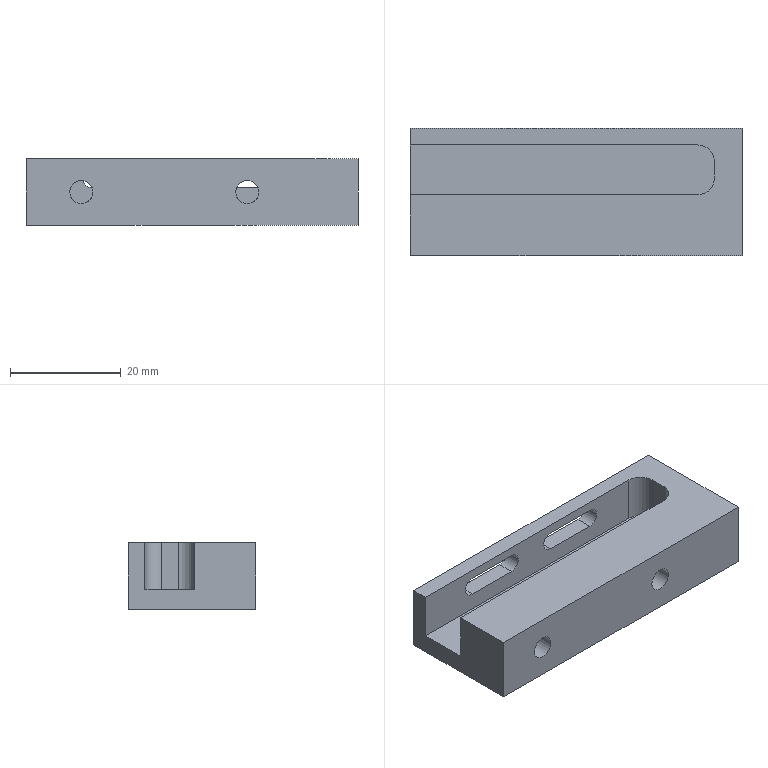Part | NX | features BREP 1 | 1 solid | 22 faces | box 60 x 23 x 12 mm | volume 11813 mm3 | plane 14 | cylinder 8 | commonest cylinder face diameters 3.5 x4 4.2 x2 6 x2
STEP:
#1=CARTESIAN_POINT('',(0.,-12.,6.));
#2=VERTEX_POINT('',#1);
#3=CARTESIAN_POINT('',(0.,-23.,6.));
#4=VERTEX_POINT('',#3);
#5=CARTESIAN_POINT('',(0.,0.,6.));
#6=DIRECTION('',(0.,-1.,0.));
#7=VECTOR('',#6,1000.);
#8=LINE('',#5,#7);
#9=EDGE_CURVE('',#2,#4,#8,.T.);
#10=ORIENTED_EDGE('',*,*,#9,.F.);
#11=CARTESIAN_POINT('',(0.,-12.,-2.5));
#12=VERTEX_POINT('',#11);
#13=CARTESIAN_POINT('',(0.,-12.,-2.5));
#14=DIRECTION('',(0.,0.,1.));
#15=VECTOR('',#14,1000.);
#16=LINE('',#13,#15);
#17=EDGE_CURVE('',#12,#2,#16,.T.);
#18=ORIENTED_EDGE('',*,*,#17,.F.);
#19=CARTESIAN_POINT('',(0.,-3.,-2.5));
#20=VERTEX_POINT('',#19);
#21=CARTESIAN_POINT('',(0.,0.,-2.5));
#22=DIRECTION('',(0.,-1.,0.));
#23=VECTOR('',#22,1000.);
#24=LINE('',#21,#23);
#25=EDGE_CURVE('',#20,#12,#24,.T.);
#26=ORIENTED_EDGE('',*,*,#25,.F.);
#27=CARTESIAN_POINT('',(0.,-3.,6.));
#28=VERTEX_POINT('',#27);
#29=CARTESIAN_POINT('',(0.,-3.,-2.5));
#30=DIRECTION('',(0.,0.,1.));
#31=VECTOR('',#30,1000.);
#32=LINE('',#29,#31);
#33=EDGE_CURVE('',#20,#28,#32,.T.);
#34=ORIENTED_EDGE('',*,*,#33,.T.);
#35=CARTESIAN_POINT('',(0.,0.,6.));
#36=VERTEX_POINT('',#35);
#37=CARTESIAN_POINT('',(0.,0.,6.));
#38=DIRECTION('',(0.,-1.,0.));
#39=VECTOR('',#38,1000.);
#40=LINE('',#37,#39);
#41=EDGE_CURVE('',#36,#28,#40,.T.);
#42=ORIENTED_EDGE('',*,*,#41,.F.);
#43=CARTESIAN_POINT('',(0.,0.,-6.));
#44=VERTEX_POINT('',#43);
#45=CARTESIAN_POINT('',(0.,0.,6.));
#46=DIRECTION('',(0.,0.,-1.));
#47=VECTOR('',#46,1000.);
#48=LINE('',#45,#47);
#49=EDGE_CURVE('',#36,#44,#48,.T.);
#50=ORIENTED_EDGE('',*,*,#49,.T.);
#51=CARTESIAN_POINT('',(0.,-23.,-6.));
#52=VERTEX_POINT('',#51);
#53=CARTESIAN_POINT('',(0.,0.,-6.));
#54=DIRECTION('',(0.,-1.,0.));
#55=VECTOR('',#54,1000.);
#56=LINE('',#53,#55);
#57=EDGE_CURVE('',#44,#52,#56,.T.);
#58=ORIENTED_EDGE('',*,*,#57,.T.);
#59=CARTESIAN_POINT('',(0.,-23.,6.));
#60=DIRECTION('',(0.,0.,-1.));
#61=VECTOR('',#60,1000.);
#62=LINE('',#59,#61);
#63=EDGE_CURVE('',#4,#52,#62,.T.);
#64=ORIENTED_EDGE('',*,*,#63,.F.);
#65=EDGE_LOOP('',(#10,#18,#26,#34,#42,#50,#58,#64));
#66=FACE_BOUND('',#65,.T.);
#67=CARTESIAN_POINT('',(0.,0.,6.));
#68=DIRECTION('',(1.,0.,0.));
#69=DIRECTION('',(0.,-1.,0.));
#70=AXIS2_PLACEMENT_3D('',#67,#68,#69);
#71=PLANE('',#70);
#72=ADVANCED_FACE('',(#66),#71,.F.);
#73=CARTESIAN_POINT('',(10.,-23.,-2.1));
#74=VERTEX_POINT('',#73);
#75=CARTESIAN_POINT('',(10.,-23.,0.));
#76=DIRECTION('',(0.,-1.,0.));
#77=DIRECTION('',(0.,0.,-1.));
#78=AXIS2_PLACEMENT_3D('',#75,#76,#77);
#79=CIRCLE('',#78,2.1);
#80=EDGE_CURVE('',#74,#74,#79,.T.);
#81=ORIENTED_EDGE('',*,*,#80,.F.);
#82=EDGE_LOOP('',(#81));
#83=FACE_BOUND('',#82,.T.);
#84=CARTESIAN_POINT('',(40.,-23.,-2.1));
#85=VERTEX_POINT('',#84);
#86=CARTESIAN_POINT('',(40.,-23.,0.));
#87=DIRECTION('',(0.,-1.,0.));
#88=DIRECTION('',(0.,0.,-1.));
#89=AXIS2_PLACEMENT_3D('',#86,#87,#88);
#90=CIRCLE('',#89,2.1);
#91=EDGE_CURVE('',#85,#85,#90,.T.);
#92=ORIENTED_EDGE('',*,*,#91,.F.);
#93=EDGE_LOOP('',(#92));
#94=FACE_BOUND('',#93,.T.);
#95=CARTESIAN_POINT('',(60.,-23.,-6.));
#96=VERTEX_POINT('',#95);
#97=CARTESIAN_POINT('',(0.,-23.,-6.));
#98=DIRECTION('',(1.,0.,0.));
#99=VECTOR('',#98,1000.);
#100=LINE('',#97,#99);
#101=EDGE_CURVE('',#52,#96,#100,.T.);
#102=ORIENTED_EDGE('',*,*,#101,.T.);
#103=CARTESIAN_POINT('',(60.,-23.,6.));
#104=VERTEX_POINT('',#103);
#105=CARTESIAN_POINT('',(60.,-23.,6.));
#106=DIRECTION('',(0.,0.,-1.));
#107=VECTOR('',#106,1000.);
#108=LINE('',#105,#107);
#109=EDGE_CURVE('',#104,#96,#108,.T.);
#110=ORIENTED_EDGE('',*,*,#109,.F.);
#111=CARTESIAN_POINT('',(0.,-23.,6.));
#112=DIRECTION('',(1.,0.,0.));
#113=VECTOR('',#112,1000.);
#114=LINE('',#111,#113);
#115=EDGE_CURVE('',#4,#104,#114,.T.);
#116=ORIENTED_EDGE('',*,*,#115,.F.);
#117=ORIENTED_EDGE('',*,*,#63,.T.);
#118=EDGE_LOOP('',(#102,#110,#116,#117));
#119=FACE_BOUND('',#118,.T.);
#120=CARTESIAN_POINT('',(0.,-23.,6.));
#121=DIRECTION('',(0.,1.,0.));
#122=DIRECTION('',(0.,0.,-1.));
#123=AXIS2_PLACEMENT_3D('',#120,#121,#122);
#124=PLANE('',#123);
#125=ADVANCED_FACE('',(#83,#94,#119),#124,.F.);
#126=CARTESIAN_POINT('',(60.,0.,-6.));
#127=VERTEX_POINT('',#126);
#128=CARTESIAN_POINT('',(60.,0.,-6.));
#129=DIRECTION('',(0.,1.,0.));
#130=VECTOR('',#129,1000.);
#131=LINE('',#128,#130);
#132=EDGE_CURVE('',#96,#127,#131,.T.);
#133=ORIENTED_EDGE('',*,*,#132,.T.);
#134=CARTESIAN_POINT('',(60.,0.,6.));
#135=VERTEX_POINT('',#134);
#136=CARTESIAN_POINT('',(60.,0.,6.));
#137=DIRECTION('',(0.,0.,-1.));
#138=VECTOR('',#137,1000.);
#139=LINE('',#136,#138);
#140=EDGE_CURVE('',#135,#127,#139,.T.);
#141=ORIENTED_EDGE('',*,*,#140,.F.);
#142=CARTESIAN_POINT('',(60.,0.,6.));
#143=DIRECTION('',(0.,1.,0.));
#144=VECTOR('',#143,1000.);
#145=LINE('',#142,#144);
#146=EDGE_CURVE('',#104,#135,#145,.T.);
#147=ORIENTED_EDGE('',*,*,#146,.F.);
#148=ORIENTED_EDGE('',*,*,#109,.T.);
#149=EDGE_LOOP('',(#133,#141,#147,#148));
#150=FACE_BOUND('',#149,.T.);
#151=CARTESIAN_POINT('',(60.,0.,6.));
#152=DIRECTION('',(-1.,0.,0.));
#153=DIRECTION('',(0.,0.,-1.));
#154=AXIS2_PLACEMENT_3D('',#151,#152,#153);
#155=PLANE('',#154);
#156=ADVANCED_FACE('',(#150),#155,.F.);
#157=CARTESIAN_POINT('',(32.,0.,0.75));
#158=VERTEX_POINT('',#157);
#159=CARTESIAN_POINT('',(32.,0.,4.25));
#160=VERTEX_POINT('',#159);
#161=CARTESIAN_POINT('',(32.,0.,2.5));
#162=DIRECTION('',(0.,1.,0.));
#163=DIRECTION('',(0.,0.,1.));
#164=AXIS2_PLACEMENT_3D('',#161,#162,#163);
#165=CIRCLE('',#164,1.75);
#166=EDGE_CURVE('',#158,#160,#165,.T.);
#167=ORIENTED_EDGE('',*,*,#166,.F.);
#168=CARTESIAN_POINT('',(42.,0.,0.75));
#169=VERTEX_POINT('',#168);
#170=CARTESIAN_POINT('',(42.,0.,0.75));
#171=DIRECTION('',(-1.,0.,0.));
#172=VECTOR('',#171,1000.);
#173=LINE('',#170,#172);
#174=EDGE_CURVE('',#169,#158,#173,.T.);
#175=ORIENTED_EDGE('',*,*,#174,.F.);
#176=CARTESIAN_POINT('',(42.,0.,4.25));
#177=VERTEX_POINT('',#176);
#178=CARTESIAN_POINT('',(42.,0.,2.5));
#179=DIRECTION('',(0.,1.,0.));
#180=DIRECTION('',(0.,0.,1.));
#181=AXIS2_PLACEMENT_3D('',#178,#179,#180);
#182=CIRCLE('',#181,1.75);
#183=EDGE_CURVE('',#177,#169,#182,.T.);
#184=ORIENTED_EDGE('',*,*,#183,.F.);
#185=CARTESIAN_POINT('',(42.,0.,4.25));
#186=DIRECTION('',(1.,0.,0.));
#187=VECTOR('',#186,1000.);
#188=LINE('',#185,#187);
#189=EDGE_CURVE('',#160,#177,#188,.T.);
#190=ORIENTED_EDGE('',*,*,#189,.F.);
#191=EDGE_LOOP('',(#167,#175,#184,#190));
#192=FACE_BOUND('',#191,.T.);
#193=CARTESIAN_POINT('',(12.,0.,0.75));
#194=VERTEX_POINT('',#193);
#195=CARTESIAN_POINT('',(12.,0.,4.25));
#196=VERTEX_POINT('',#195);
#197=CARTESIAN_POINT('',(12.,0.,2.5));
#198=DIRECTION('',(0.,1.,0.));
#199=DIRECTION('',(0.,0.,1.));
#200=AXIS2_PLACEMENT_3D('',#197,#198,#199);
#201=CIRCLE('',#200,1.75);
#202=EDGE_CURVE('',#194,#196,#201,.T.);
#203=ORIENTED_EDGE('',*,*,#202,.F.);
#204=CARTESIAN_POINT('',(22.,0.,0.75));
#205=VERTEX_POINT('',#204);
#206=CARTESIAN_POINT('',(22.,0.,0.75));
#207=DIRECTION('',(-1.,0.,0.));
#208=VECTOR('',#207,1000.);
#209=LINE('',#206,#208);
#210=EDGE_CURVE('',#205,#194,#209,.T.);
#211=ORIENTED_EDGE('',*,*,#210,.F.);
#212=CARTESIAN_POINT('',(22.,0.,4.25));
#213=VERTEX_POINT('',#212);
#214=CARTESIAN_POINT('',(22.,0.,2.5));
#215=DIRECTION('',(0.,1.,0.));
#216=DIRECTION('',(0.,0.,1.));
#217=AXIS2_PLACEMENT_3D('',#214,#215,#216);
#218=CIRCLE('',#217,1.75);
#219=EDGE_CURVE('',#213,#205,#218,.T.);
#220=ORIENTED_EDGE('',*,*,#219,.F.);
#221=CARTESIAN_POINT('',(22.,0.,4.25));
#222=DIRECTION('',(1.,0.,0.));
#223=VECTOR('',#222,1000.);
#224=LINE('',#221,#223);
#225=EDGE_CURVE('',#196,#213,#224,.T.);
#226=ORIENTED_EDGE('',*,*,#225,.F.);
#227=EDGE_LOOP('',(#203,#211,#220,#226));
#228=FACE_BOUND('',#227,.T.);
#229=CARTESIAN_POINT('',(0.,0.,-6.));
#230=DIRECTION('',(-1.,0.,0.));
#231=VECTOR('',#230,1000.);
#232=LINE('',#229,#231);
#233=EDGE_CURVE('',#127,#44,#232,.T.);
#234=ORIENTED_EDGE('',*,*,#233,.T.);
#235=ORIENTED_EDGE('',*,*,#49,.F.);
#236=CARTESIAN_POINT('',(0.,0.,6.));
#237=DIRECTION('',(-1.,0.,0.));
#238=VECTOR('',#237,1000.);
#239=LINE('',#236,#238);
#240=EDGE_CURVE('',#135,#36,#239,.T.);
#241=ORIENTED_EDGE('',*,*,#240,.F.);
#242=ORIENTED_EDGE('',*,*,#140,.T.);
#243=EDGE_LOOP('',(#234,#235,#241,#242));
#244=FACE_BOUND('',#243,.T.);
#245=CARTESIAN_POINT('',(0.,0.,6.));
#246=DIRECTION('',(0.,-1.,0.));
#247=DIRECTION('',(0.,0.,1.));
#248=AXIS2_PLACEMENT_3D('',#245,#246,#247);
#249=PLANE('',#248);
#250=ADVANCED_FACE('',(#192,#228,#244),#249,.F.);
#251=CARTESIAN_POINT('',(52.,-12.,6.));
#252=VERTEX_POINT('',#251);
#253=CARTESIAN_POINT('',(0.,-12.,6.));
#254=DIRECTION('',(1.,0.,0.));
#255=VECTOR('',#254,1000.);
#256=LINE('',#253,#255);
#257=EDGE_CURVE('',#2,#252,#256,.T.);
#258=ORIENTED_EDGE('',*,*,#257,.F.);
#259=ORIENTED_EDGE('',*,*,#9,.T.);
#260=ORIENTED_EDGE('',*,*,#115,.T.);
#261=ORIENTED_EDGE('',*,*,#146,.T.);
#262=ORIENTED_EDGE('',*,*,#240,.T.);
#263=ORIENTED_EDGE('',*,*,#41,.T.);
#264=CARTESIAN_POINT('',(52.,-3.,6.));
#265=VERTEX_POINT('',#264);
#266=CARTESIAN_POINT('',(0.,-3.,6.));
#267=DIRECTION('',(1.,0.,0.));
#268=VECTOR('',#267,1000.);
#269=LINE('',#266,#268);
#270=EDGE_CURVE('',#28,#265,#269,.T.);
#271=ORIENTED_EDGE('',*,*,#270,.T.);
#272=CARTESIAN_POINT('',(55.,-6.,6.));
#273=VERTEX_POINT('',#272);
#274=CARTESIAN_POINT('',(52.,-6.,6.));
#275=DIRECTION('',(0.,0.,-1.));
#276=DIRECTION('',(1.,0.,0.));
#277=AXIS2_PLACEMENT_3D('',#274,#275,#276);
#278=CIRCLE('',#277,3.);
#279=EDGE_CURVE('',#265,#273,#278,.T.);
#280=ORIENTED_EDGE('',*,*,#279,.T.);
#281=CARTESIAN_POINT('',(55.,-9.,6.));
#282=VERTEX_POINT('',#281);
#283=CARTESIAN_POINT('',(55.,0.,6.));
#284=DIRECTION('',(0.,-1.,0.));
#285=VECTOR('',#284,1000.);
#286=LINE('',#283,#285);
#287=EDGE_CURVE('',#273,#282,#286,.T.);
#288=ORIENTED_EDGE('',*,*,#287,.T.);
#289=CARTESIAN_POINT('',(52.,-9.,6.));
#290=DIRECTION('',(0.,0.,-1.));
#291=DIRECTION('',(1.,0.,0.));
#292=AXIS2_PLACEMENT_3D('',#289,#290,#291);
#293=CIRCLE('',#292,3.);
#294=EDGE_CURVE('',#282,#252,#293,.T.);
#295=ORIENTED_EDGE('',*,*,#294,.T.);
#296=EDGE_LOOP('',(#258,#259,#260,#261,#262,#263,#271,#280,#288,#295));
#297=FACE_BOUND('',#296,.T.);
#298=CARTESIAN_POINT('',(0.,0.,6.));
#299=DIRECTION('',(0.,0.,1.));
#300=DIRECTION('',(-1.,0.,0.));
#301=AXIS2_PLACEMENT_3D('',#298,#299,#300);
#302=PLANE('',#301);
#303=ADVANCED_FACE('',(#297),#302,.T.);
#304=ORIENTED_EDGE('',*,*,#57,.F.);
#305=ORIENTED_EDGE('',*,*,#233,.F.);
#306=ORIENTED_EDGE('',*,*,#132,.F.);
#307=ORIENTED_EDGE('',*,*,#101,.F.);
#308=EDGE_LOOP('',(#304,#305,#306,#307));
#309=FACE_BOUND('',#308,.T.);
#310=CARTESIAN_POINT('',(0.,0.,-6.));
#311=DIRECTION('',(0.,0.,1.));
#312=DIRECTION('',(-1.,0.,0.));
#313=AXIS2_PLACEMENT_3D('',#310,#311,#312);
#314=PLANE('',#313);
#315=ADVANCED_FACE('',(#309),#314,.F.);
#316=CARTESIAN_POINT('',(55.,-6.,-2.5));
#317=VERTEX_POINT('',#316);
#318=CARTESIAN_POINT('',(55.,-9.,-2.5));
#319=VERTEX_POINT('',#318);
#320=CARTESIAN_POINT('',(55.,0.,-2.5));
#321=DIRECTION('',(0.,-1.,0.));
#322=VECTOR('',#321,1000.);
#323=LINE('',#320,#322);
#324=EDGE_CURVE('',#317,#319,#323,.T.);
#325=ORIENTED_EDGE('',*,*,#324,.T.);
#326=CARTESIAN_POINT('',(55.,-9.,-2.5));
#327=DIRECTION('',(0.,0.,1.));
#328=VECTOR('',#327,1000.);
#329=LINE('',#326,#328);
#330=EDGE_CURVE('',#319,#282,#329,.T.);
#331=ORIENTED_EDGE('',*,*,#330,.T.);
#332=ORIENTED_EDGE('',*,*,#287,.F.);
#333=CARTESIAN_POINT('',(55.,-6.,-2.5));
#334=DIRECTION('',(0.,0.,-1.));
#335=VECTOR('',#334,1000.);
#336=LINE('',#333,#335);
#337=EDGE_CURVE('',#273,#317,#336,.T.);
#338=ORIENTED_EDGE('',*,*,#337,.T.);
#339=EDGE_LOOP('',(#325,#331,#332,#338));
#340=FACE_BOUND('',#339,.T.);
#341=CARTESIAN_POINT('',(55.,0.,-2.5));
#342=DIRECTION('',(-1.,0.,0.));
#343=DIRECTION('',(0.,1.,0.));
#344=AXIS2_PLACEMENT_3D('',#341,#342,#343);
#345=PLANE('',#344);
#346=ADVANCED_FACE('',(#340),#345,.T.);
#347=CARTESIAN_POINT('',(12.1,-12.,0.));
#348=VERTEX_POINT('',#347);
#349=CARTESIAN_POINT('',(10.,-12.,0.));
#350=DIRECTION('',(0.,-1.,0.));
#351=DIRECTION('',(1.,0.,0.));
#352=AXIS2_PLACEMENT_3D('',#349,#350,#351);
#353=CIRCLE('',#352,2.1);
#354=EDGE_CURVE('',#348,#348,#353,.T.);
#355=ORIENTED_EDGE('',*,*,#354,.T.);
#356=EDGE_LOOP('',(#355));
#357=FACE_BOUND('',#356,.T.);
#358=CARTESIAN_POINT('',(42.1,-12.,0.));
#359=VERTEX_POINT('',#358);
#360=CARTESIAN_POINT('',(40.,-12.,0.));
#361=DIRECTION('',(0.,-1.,0.));
#362=DIRECTION('',(1.,0.,0.));
#363=AXIS2_PLACEMENT_3D('',#360,#361,#362);
#364=CIRCLE('',#363,2.1);
#365=EDGE_CURVE('',#359,#359,#364,.T.);
#366=ORIENTED_EDGE('',*,*,#365,.T.);
#367=EDGE_LOOP('',(#366));
#368=FACE_BOUND('',#367,.T.);
#369=ORIENTED_EDGE('',*,*,#257,.T.);
#370=CARTESIAN_POINT('',(52.,-12.,-2.5));
#371=VERTEX_POINT('',#370);
#372=CARTESIAN_POINT('',(52.,-12.,-2.5));
#373=DIRECTION('',(0.,0.,-1.));
#374=VECTOR('',#373,1000.);
#375=LINE('',#372,#374);
#376=EDGE_CURVE('',#252,#371,#375,.T.);
#377=ORIENTED_EDGE('',*,*,#376,.T.);
#378=CARTESIAN_POINT('',(0.,-12.,-2.5));
#379=DIRECTION('',(1.,0.,0.));
#380=VECTOR('',#379,1000.);
#381=LINE('',#378,#380);
#382=EDGE_CURVE('',#12,#371,#381,.T.);
#383=ORIENTED_EDGE('',*,*,#382,.F.);
#384=ORIENTED_EDGE('',*,*,#17,.T.);
#385=EDGE_LOOP('',(#369,#377,#383,#384));
#386=FACE_BOUND('',#385,.T.);
#387=CARTESIAN_POINT('',(0.,-12.,-2.5));
#388=DIRECTION('',(0.,-1.,0.));
#389=DIRECTION('',(-1.,0.,0.));
#390=AXIS2_PLACEMENT_3D('',#387,#388,#389);
#391=PLANE('',#390);
#392=ADVANCED_FACE('',(#357,#368,#386),#391,.F.);
#393=CARTESIAN_POINT('',(42.,-3.,0.75));
#394=VERTEX_POINT('',#393);
#395=CARTESIAN_POINT('',(32.,-3.,0.75));
#396=VERTEX_POINT('',#395);
#397=CARTESIAN_POINT('',(42.,-3.,0.75));
#398=DIRECTION('',(-1.,0.,0.));
#399=VECTOR('',#398,1000.);
#400=LINE('',#397,#399);
#401=EDGE_CURVE('',#394,#396,#400,.T.);
#402=ORIENTED_EDGE('',*,*,#401,.T.);
#403=CARTESIAN_POINT('',(32.,-3.,4.25));
#404=VERTEX_POINT('',#403);
#405=CARTESIAN_POINT('',(32.,-3.,2.5));
#406=DIRECTION('',(0.,1.,0.));
#407=DIRECTION('',(1.,0.,0.));
#408=AXIS2_PLACEMENT_3D('',#405,#406,#407);
#409=CIRCLE('',#408,1.75);
#410=EDGE_CURVE('',#396,#404,#409,.T.);
#411=ORIENTED_EDGE('',*,*,#410,.T.);
#412=CARTESIAN_POINT('',(42.,-3.,4.25));
#413=VERTEX_POINT('',#412);
#414=CARTESIAN_POINT('',(42.,-3.,4.25));
#415=DIRECTION('',(1.,0.,0.));
#416=VECTOR('',#415,1000.);
#417=LINE('',#414,#416);
#418=EDGE_CURVE('',#404,#413,#417,.T.);
#419=ORIENTED_EDGE('',*,*,#418,.T.);
#420=CARTESIAN_POINT('',(42.,-3.,2.5));
#421=DIRECTION('',(0.,1.,0.));
#422=DIRECTION('',(1.,0.,0.));
#423=AXIS2_PLACEMENT_3D('',#420,#421,#422);
#424=CIRCLE('',#423,1.75);
#425=EDGE_CURVE('',#413,#394,#424,.T.);
#426=ORIENTED_EDGE('',*,*,#425,.T.);
#427=EDGE_LOOP('',(#402,#411,#419,#426));
#428=FACE_BOUND('',#427,.T.);
#429=CARTESIAN_POINT('',(22.,-3.,0.75));
#430=VERTEX_POINT('',#429);
#431=CARTESIAN_POINT('',(12.,-3.,0.75));
#432=VERTEX_POINT('',#431);
#433=CARTESIAN_POINT('',(22.,-3.,0.75));
#434=DIRECTION('',(-1.,0.,0.));
#435=VECTOR('',#434,1000.);
#436=LINE('',#433,#435);
#437=EDGE_CURVE('',#430,#432,#436,.T.);
#438=ORIENTED_EDGE('',*,*,#437,.T.);
#439=CARTESIAN_POINT('',(12.,-3.,4.25));
#440=VERTEX_POINT('',#439);
#441=CARTESIAN_POINT('',(12.,-3.,2.5));
#442=DIRECTION('',(0.,1.,0.));
#443=DIRECTION('',(1.,0.,0.));
#444=AXIS2_PLACEMENT_3D('',#441,#442,#443);
#445=CIRCLE('',#444,1.75);
#446=EDGE_CURVE('',#432,#440,#445,.T.);
#447=ORIENTED_EDGE('',*,*,#446,.T.);
#448=CARTESIAN_POINT('',(22.,-3.,4.25));
#449=VERTEX_POINT('',#448);
#450=CARTESIAN_POINT('',(22.,-3.,4.25));
#451=DIRECTION('',(1.,0.,0.));
#452=VECTOR('',#451,1000.);
#453=LINE('',#450,#452);
#454=EDGE_CURVE('',#440,#449,#453,.T.);
#455=ORIENTED_EDGE('',*,*,#454,.T.);
#456=CARTESIAN_POINT('',(22.,-3.,2.5));
#457=DIRECTION('',(0.,1.,0.));
#458=DIRECTION('',(1.,0.,0.));
#459=AXIS2_PLACEMENT_3D('',#456,#457,#458);
#460=CIRCLE('',#459,1.75);
#461=EDGE_CURVE('',#449,#430,#460,.T.);
#462=ORIENTED_EDGE('',*,*,#461,.T.);
#463=EDGE_LOOP('',(#438,#447,#455,#462));
#464=FACE_BOUND('',#463,.T.);
#465=CARTESIAN_POINT('',(52.,-3.,-2.5));
#466=VERTEX_POINT('',#465);
#467=CARTESIAN_POINT('',(0.,-3.,-2.5));
#468=DIRECTION('',(1.,0.,0.));
#469=VECTOR('',#468,1000.);
#470=LINE('',#467,#469);
#471=EDGE_CURVE('',#20,#466,#470,.T.);
#472=ORIENTED_EDGE('',*,*,#471,.T.);
#473=CARTESIAN_POINT('',(52.,-3.,6.));
#474=DIRECTION('',(0.,0.,1.));
#475=VECTOR('',#474,1000.);
#476=LINE('',#473,#475);
#477=EDGE_CURVE('',#466,#265,#476,.T.);
#478=ORIENTED_EDGE('',*,*,#477,.T.);
#479=ORIENTED_EDGE('',*,*,#270,.F.);
#480=ORIENTED_EDGE('',*,*,#33,.F.);
#481=EDGE_LOOP('',(#472,#478,#479,#480));
#482=FACE_BOUND('',#481,.T.);
#483=CARTESIAN_POINT('',(0.,-3.,-2.5));
#484=DIRECTION('',(0.,-1.,0.));
#485=DIRECTION('',(-1.,0.,0.));
#486=AXIS2_PLACEMENT_3D('',#483,#484,#485);
#487=PLANE('',#486);
#488=ADVANCED_FACE('',(#428,#464,#482),#487,.T.);
#489=ORIENTED_EDGE('',*,*,#382,.T.);
#490=CARTESIAN_POINT('',(52.,-9.,-2.5));
#491=DIRECTION('',(0.,0.,1.));
#492=DIRECTION('',(1.,0.,0.));
#493=AXIS2_PLACEMENT_3D('',#490,#491,#492);
#494=CIRCLE('',#493,3.);
#495=EDGE_CURVE('',#371,#319,#494,.T.);
#496=ORIENTED_EDGE('',*,*,#495,.T.);
#497=ORIENTED_EDGE('',*,*,#324,.F.);
#498=CARTESIAN_POINT('',(52.,-6.,-2.5));
#499=DIRECTION('',(0.,0.,1.));
#500=DIRECTION('',(1.,0.,0.));
#501=AXIS2_PLACEMENT_3D('',#498,#499,#500);
#502=CIRCLE('',#501,3.);
#503=EDGE_CURVE('',#317,#466,#502,.T.);
#504=ORIENTED_EDGE('',*,*,#503,.T.);
#505=ORIENTED_EDGE('',*,*,#471,.F.);
#506=ORIENTED_EDGE('',*,*,#25,.T.);
#507=EDGE_LOOP('',(#489,#496,#497,#504,#505,#506));
#508=FACE_BOUND('',#507,.T.);
#509=CARTESIAN_POINT('',(0.,0.,-2.5));
#510=DIRECTION('',(0.,0.,1.));
#511=DIRECTION('',(-1.,0.,0.));
#512=AXIS2_PLACEMENT_3D('',#509,#510,#511);
#513=PLANE('',#512);
#514=ADVANCED_FACE('',(#508),#513,.T.);
#515=ORIENTED_EDGE('',*,*,#495,.F.);
#516=ORIENTED_EDGE('',*,*,#376,.F.);
#517=ORIENTED_EDGE('',*,*,#294,.F.);
#518=ORIENTED_EDGE('',*,*,#330,.F.);
#519=EDGE_LOOP('',(#515,#516,#517,#518));
#520=FACE_BOUND('',#519,.T.);
#521=CARTESIAN_POINT('',(52.,-9.,-2.5));
#522=DIRECTION('',(0.,0.,1.));
#523=DIRECTION('',(-1.,0.,0.));
#524=AXIS2_PLACEMENT_3D('',#521,#522,#523);
#525=CYLINDRICAL_SURFACE('',#524,3.);
#526=ADVANCED_FACE('',(#520),#525,.F.);
#527=ORIENTED_EDGE('',*,*,#503,.F.);
#528=ORIENTED_EDGE('',*,*,#337,.F.);
#529=ORIENTED_EDGE('',*,*,#279,.F.);
#530=ORIENTED_EDGE('',*,*,#477,.F.);
#531=EDGE_LOOP('',(#527,#528,#529,#530));
#532=FACE_BOUND('',#531,.T.);
#533=CARTESIAN_POINT('',(52.,-6.,-2.5));
#534=DIRECTION('',(0.,0.,-1.));
#535=DIRECTION('',(1.,0.,0.));
#536=AXIS2_PLACEMENT_3D('',#533,#534,#535);
#537=CYLINDRICAL_SURFACE('',#536,3.);
#538=ADVANCED_FACE('',(#532),#537,.F.);
#539=CARTESIAN_POINT('',(22.,-16.946,0.75));
#540=DIRECTION('',(0.,1.,0.));
#541=VECTOR('',#540,1000.);
#542=LINE('',#539,#541);
#543=EDGE_CURVE('',#430,#205,#542,.T.);
#544=ORIENTED_EDGE('',*,*,#543,.T.);
#545=ORIENTED_EDGE('',*,*,#210,.T.);
#546=CARTESIAN_POINT('',(12.,-16.946,0.75));
#547=DIRECTION('',(0.,1.,0.));
#548=VECTOR('',#547,1000.);
#549=LINE('',#546,#548);
#550=EDGE_CURVE('',#432,#194,#549,.T.);
#551=ORIENTED_EDGE('',*,*,#550,.F.);
#552=ORIENTED_EDGE('',*,*,#437,.F.);
#553=EDGE_LOOP('',(#544,#545,#551,#552));
#554=FACE_BOUND('',#553,.T.);
#555=CARTESIAN_POINT('',(22.,-16.946,0.75));
#556=DIRECTION('',(0.,0.,-1.));
#557=DIRECTION('',(1.,0.,0.));
#558=AXIS2_PLACEMENT_3D('',#555,#556,#557);
#559=PLANE('',#558);
#560=ADVANCED_FACE('',(#554),#559,.F.);
#561=ORIENTED_EDGE('',*,*,#550,.T.);
#562=ORIENTED_EDGE('',*,*,#202,.T.);
#563=CARTESIAN_POINT('',(12.,-16.946,4.25));
#564=DIRECTION('',(0.,1.,0.));
#565=VECTOR('',#564,1000.);
#566=LINE('',#563,#565);
#567=EDGE_CURVE('',#440,#196,#566,.T.);
#568=ORIENTED_EDGE('',*,*,#567,.F.);
#569=ORIENTED_EDGE('',*,*,#446,.F.);
#570=EDGE_LOOP('',(#561,#562,#568,#569));
#571=FACE_BOUND('',#570,.T.);
#572=CARTESIAN_POINT('',(12.,-16.946,2.5));
#573=DIRECTION('',(0.,1.,0.));
#574=DIRECTION('',(0.,0.,-1.));
#575=AXIS2_PLACEMENT_3D('',#572,#573,#574);
#576=CYLINDRICAL_SURFACE('',#575,1.75);
#577=ADVANCED_FACE('',(#571),#576,.F.);
#578=ORIENTED_EDGE('',*,*,#567,.T.);
#579=ORIENTED_EDGE('',*,*,#225,.T.);
#580=CARTESIAN_POINT('',(22.,-16.946,4.25));
#581=DIRECTION('',(0.,1.,0.));
#582=VECTOR('',#581,1000.);
#583=LINE('',#580,#582);
#584=EDGE_CURVE('',#449,#213,#583,.T.);
#585=ORIENTED_EDGE('',*,*,#584,.F.);
#586=ORIENTED_EDGE('',*,*,#454,.F.);
#587=EDGE_LOOP('',(#578,#579,#585,#586));
#588=FACE_BOUND('',#587,.T.);
#589=CARTESIAN_POINT('',(22.,-16.946,4.25));
#590=DIRECTION('',(0.,0.,1.));
#591=DIRECTION('',(-1.,0.,0.));
#592=AXIS2_PLACEMENT_3D('',#589,#590,#591);
#593=PLANE('',#592);
#594=ADVANCED_FACE('',(#588),#593,.F.);
#595=ORIENTED_EDGE('',*,*,#584,.T.);
#596=ORIENTED_EDGE('',*,*,#219,.T.);
#597=ORIENTED_EDGE('',*,*,#543,.F.);
#598=ORIENTED_EDGE('',*,*,#461,.F.);
#599=EDGE_LOOP('',(#595,#596,#597,#598));
#600=FACE_BOUND('',#599,.T.);
#601=CARTESIAN_POINT('',(22.,-16.946,2.5));
#602=DIRECTION('',(0.,1.,0.));
#603=DIRECTION('',(0.,0.,-1.));
#604=AXIS2_PLACEMENT_3D('',#601,#602,#603);
#605=CYLINDRICAL_SURFACE('',#604,1.75);
#606=ADVANCED_FACE('',(#600),#605,.F.);
#607=CARTESIAN_POINT('',(42.,-16.946,0.75));
#608=DIRECTION('',(0.,1.,0.));
#609=VECTOR('',#608,1000.);
#610=LINE('',#607,#609);
#611=EDGE_CURVE('',#394,#169,#610,.T.);
#612=ORIENTED_EDGE('',*,*,#611,.T.);
#613=ORIENTED_EDGE('',*,*,#174,.T.);
#614=CARTESIAN_POINT('',(32.,-16.946,0.75));
#615=DIRECTION('',(0.,1.,0.));
#616=VECTOR('',#615,1000.);
#617=LINE('',#614,#616);
#618=EDGE_CURVE('',#396,#158,#617,.T.);
#619=ORIENTED_EDGE('',*,*,#618,.F.);
#620=ORIENTED_EDGE('',*,*,#401,.F.);
#621=EDGE_LOOP('',(#612,#613,#619,#620));
#622=FACE_BOUND('',#621,.T.);
#623=CARTESIAN_POINT('',(42.,-16.946,0.75));
#624=DIRECTION('',(0.,0.,-1.));
#625=DIRECTION('',(1.,0.,0.));
#626=AXIS2_PLACEMENT_3D('',#623,#624,#625);
#627=PLANE('',#626);
#628=ADVANCED_FACE('',(#622),#627,.F.);
#629=ORIENTED_EDGE('',*,*,#618,.T.);
#630=ORIENTED_EDGE('',*,*,#166,.T.);
#631=CARTESIAN_POINT('',(32.,-16.946,4.25));
#632=DIRECTION('',(0.,1.,0.));
#633=VECTOR('',#632,1000.);
#634=LINE('',#631,#633);
#635=EDGE_CURVE('',#404,#160,#634,.T.);
#636=ORIENTED_EDGE('',*,*,#635,.F.);
#637=ORIENTED_EDGE('',*,*,#410,.F.);
#638=EDGE_LOOP('',(#629,#630,#636,#637));
#639=FACE_BOUND('',#638,.T.);
#640=CARTESIAN_POINT('',(32.,-16.946,2.5));
#641=DIRECTION('',(0.,1.,0.));
#642=DIRECTION('',(0.,0.,-1.));
#643=AXIS2_PLACEMENT_3D('',#640,#641,#642);
#644=CYLINDRICAL_SURFACE('',#643,1.75);
#645=ADVANCED_FACE('',(#639),#644,.F.);
#646=ORIENTED_EDGE('',*,*,#635,.T.);
#647=ORIENTED_EDGE('',*,*,#189,.T.);
#648=CARTESIAN_POINT('',(42.,-16.946,4.25));
#649=DIRECTION('',(0.,1.,0.));
#650=VECTOR('',#649,1000.);
#651=LINE('',#648,#650);
#652=EDGE_CURVE('',#413,#177,#651,.T.);
#653=ORIENTED_EDGE('',*,*,#652,.F.);
#654=ORIENTED_EDGE('',*,*,#418,.F.);
#655=EDGE_LOOP('',(#646,#647,#653,#654));
#656=FACE_BOUND('',#655,.T.);
#657=CARTESIAN_POINT('',(42.,-16.946,4.25));
#658=DIRECTION('',(0.,0.,1.));
#659=DIRECTION('',(-1.,0.,0.));
#660=AXIS2_PLACEMENT_3D('',#657,#658,#659);
#661=PLANE('',#660);
#662=ADVANCED_FACE('',(#656),#661,.F.);
#663=ORIENTED_EDGE('',*,*,#652,.T.);
#664=ORIENTED_EDGE('',*,*,#183,.T.);
#665=ORIENTED_EDGE('',*,*,#611,.F.);
#666=ORIENTED_EDGE('',*,*,#425,.F.);
#667=EDGE_LOOP('',(#663,#664,#665,#666));
#668=FACE_BOUND('',#667,.T.);
#669=CARTESIAN_POINT('',(42.,-16.946,2.5));
#670=DIRECTION('',(0.,1.,0.));
#671=DIRECTION('',(0.,0.,-1.));
#672=AXIS2_PLACEMENT_3D('',#669,#670,#671);
#673=CYLINDRICAL_SURFACE('',#672,1.75);
#674=ADVANCED_FACE('',(#668),#673,.F.);
#675=ORIENTED_EDGE('',*,*,#91,.T.);
#676=EDGE_LOOP('',(#675));
#677=FACE_BOUND('',#676,.T.);
#678=ORIENTED_EDGE('',*,*,#365,.F.);
#679=EDGE_LOOP('',(#678));
#680=FACE_BOUND('',#679,.T.);
#681=CARTESIAN_POINT('',(40.,-23.,0.));
#682=DIRECTION('',(0.,-1.,0.));
#683=DIRECTION('',(0.,0.,1.));
#684=AXIS2_PLACEMENT_3D('',#681,#682,#683);
#685=CYLINDRICAL_SURFACE('',#684,2.1);
#686=ADVANCED_FACE('',(#677,#680),#685,.F.);
#687=ORIENTED_EDGE('',*,*,#80,.T.);
#688=EDGE_LOOP('',(#687));
#689=FACE_BOUND('',#688,.T.);
#690=ORIENTED_EDGE('',*,*,#354,.F.);
#691=EDGE_LOOP('',(#690));
#692=FACE_BOUND('',#691,.T.);
#693=CARTESIAN_POINT('',(10.,-23.,0.));
#694=DIRECTION('',(0.,-1.,0.));
#695=DIRECTION('',(0.,0.,1.));
#696=AXIS2_PLACEMENT_3D('',#693,#694,#695);
#697=CYLINDRICAL_SURFACE('',#696,2.1);
#698=ADVANCED_FACE('',(#689,#692),#697,.F.);
#699=CLOSED_SHELL('',(#72,#125,#156,#250,#303,#315,#346,#392,#488,#514,#526,#538,#560,#577,#594,#606,#628,#645,#662,#674,#686,#698));
#700=MANIFOLD_SOLID_BREP('',#699);
#701=(LENGTH_UNIT()NAMED_UNIT(*)SI_UNIT(.MILLI.,.METRE.));
#702=UNCERTAINTY_MEASURE_WITH_UNIT(LENGTH_MEASURE(0.00001),#701,'','');
#703=(NAMED_UNIT(*)PLANE_ANGLE_UNIT()SI_UNIT($,.RADIAN.));
#704=(NAMED_UNIT(*)SI_UNIT($,.STERADIAN.)SOLID_ANGLE_UNIT());
#705=(GEOMETRIC_REPRESENTATION_CONTEXT(3)GLOBAL_UNCERTAINTY_ASSIGNED_CONTEXT((#702))GLOBAL_UNIT_ASSIGNED_CONTEXT((#701,#703,#704))REPRESENTATION_CONTEXT('',''));
#706=ADVANCED_BREP_SHAPE_REPRESENTATION('',(#700),#705);